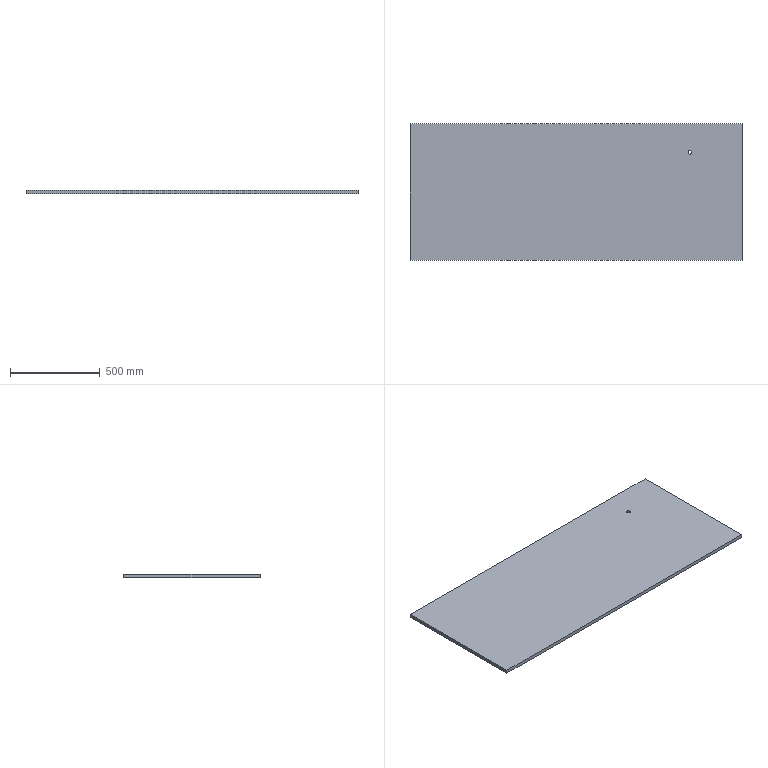Part | SolidWorks | features Extrusion 1 | 1 solid | 8 faces | box 1845 x 760 x 20 mm | volume 28037717 mm3 | plane 6 | cylinder 2 | commonest cylinder face diameters 20 x2
STEP:
#1=CARTESIAN_POINT('',(1545.,600.,20.));
#2=VERTEX_POINT('',#1);
#3=CARTESIAN_POINT('',(1565.,600.,20.));
#4=VERTEX_POINT('',#3);
#5=CARTESIAN_POINT('',(1555.,600.,20.));
#6=DIRECTION('',(0.,0.,1.));
#7=DIRECTION('',(1.,0.,0.));
#8=AXIS2_PLACEMENT_3D('',#5,#6,#7);
#9=CIRCLE('',#8,10.);
#10=EDGE_CURVE('',#2,#4,#9,.T.);
#11=ORIENTED_EDGE('',*,*,#10,.T.);
#12=CARTESIAN_POINT('',(1565.,600.,0.));
#13=VERTEX_POINT('',#12);
#14=CARTESIAN_POINT('',(1565.,600.,20.));
#15=DIRECTION('',(0.,0.,-1.));
#16=VECTOR('',#15,1000.);
#17=LINE('',#14,#16);
#18=EDGE_CURVE('',#4,#13,#17,.T.);
#19=ORIENTED_EDGE('',*,*,#18,.T.);
#20=CARTESIAN_POINT('',(1545.,600.,0.));
#21=VERTEX_POINT('',#20);
#22=CARTESIAN_POINT('',(1555.,600.,0.));
#23=DIRECTION('',(0.,0.,1.));
#24=DIRECTION('',(1.,0.,0.));
#25=AXIS2_PLACEMENT_3D('',#22,#23,#24);
#26=CIRCLE('',#25,10.);
#27=EDGE_CURVE('',#21,#13,#26,.T.);
#28=ORIENTED_EDGE('',*,*,#27,.F.);
#29=CARTESIAN_POINT('',(1545.,600.,20.));
#30=DIRECTION('',(0.,0.,-1.));
#31=VECTOR('',#30,1000.);
#32=LINE('',#29,#31);
#33=EDGE_CURVE('',#2,#21,#32,.T.);
#34=ORIENTED_EDGE('',*,*,#33,.F.);
#35=EDGE_LOOP('',(#11,#19,#28,#34));
#36=FACE_OUTER_BOUND('',#35,.T.);
#37=CARTESIAN_POINT('',(1555.,600.,20.));
#38=DIRECTION('',(0.,0.,-1.));
#39=DIRECTION('',(-1.,0.,0.));
#40=AXIS2_PLACEMENT_3D('',#37,#38,#39);
#41=CYLINDRICAL_SURFACE('',#40,10.);
#42=ADVANCED_FACE('',(#36),#41,.F.);
#43=CARTESIAN_POINT('',(0.,760.,20.));
#44=VERTEX_POINT('',#43);
#45=CARTESIAN_POINT('',(0.,0.,20.));
#46=VERTEX_POINT('',#45);
#47=CARTESIAN_POINT('',(0.,0.,20.));
#48=DIRECTION('',(0.,-1.,0.));
#49=VECTOR('',#48,1000.);
#50=LINE('',#47,#49);
#51=EDGE_CURVE('',#44,#46,#50,.T.);
#52=ORIENTED_EDGE('',*,*,#51,.T.);
#53=CARTESIAN_POINT('',(1845.,0.,20.));
#54=VERTEX_POINT('',#53);
#55=CARTESIAN_POINT('',(0.,0.,20.));
#56=DIRECTION('',(1.,0.,0.));
#57=VECTOR('',#56,1000.);
#58=LINE('',#55,#57);
#59=EDGE_CURVE('',#46,#54,#58,.T.);
#60=ORIENTED_EDGE('',*,*,#59,.T.);
#61=CARTESIAN_POINT('',(1845.,760.,20.));
#62=VERTEX_POINT('',#61);
#63=CARTESIAN_POINT('',(1845.,0.,20.));
#64=DIRECTION('',(0.,1.,0.));
#65=VECTOR('',#64,1000.);
#66=LINE('',#63,#65);
#67=EDGE_CURVE('',#54,#62,#66,.T.);
#68=ORIENTED_EDGE('',*,*,#67,.T.);
#69=CARTESIAN_POINT('',(0.,760.,20.));
#70=DIRECTION('',(-1.,0.,0.));
#71=VECTOR('',#70,1000.);
#72=LINE('',#69,#71);
#73=EDGE_CURVE('',#62,#44,#72,.T.);
#74=ORIENTED_EDGE('',*,*,#73,.T.);
#75=EDGE_LOOP('',(#52,#60,#68,#74));
#76=FACE_OUTER_BOUND('',#75,.T.);
#77=ORIENTED_EDGE('',*,*,#10,.F.);
#78=CARTESIAN_POINT('',(1555.,600.,20.));
#79=DIRECTION('',(0.,0.,1.));
#80=DIRECTION('',(1.,0.,0.));
#81=AXIS2_PLACEMENT_3D('',#78,#79,#80);
#82=CIRCLE('',#81,10.);
#83=EDGE_CURVE('',#4,#2,#82,.T.);
#84=ORIENTED_EDGE('',*,*,#83,.F.);
#85=EDGE_LOOP('',(#77,#84));
#86=FACE_BOUND('',#85,.T.);
#87=CARTESIAN_POINT('',(0.,0.,20.));
#88=DIRECTION('',(0.,0.,-1.));
#89=DIRECTION('',(-1.,0.,0.));
#90=AXIS2_PLACEMENT_3D('',#87,#88,#89);
#91=PLANE('',#90);
#92=ADVANCED_FACE('',(#76,#86),#91,.F.);
#93=CARTESIAN_POINT('',(0.,760.,0.));
#94=VERTEX_POINT('',#93);
#95=CARTESIAN_POINT('',(0.,0.,0.));
#96=VERTEX_POINT('',#95);
#97=CARTESIAN_POINT('',(0.,0.,0.));
#98=DIRECTION('',(0.,-1.,0.));
#99=VECTOR('',#98,1000.);
#100=LINE('',#97,#99);
#101=EDGE_CURVE('',#94,#96,#100,.T.);
#102=ORIENTED_EDGE('',*,*,#101,.F.);
#103=CARTESIAN_POINT('',(1845.,760.,0.));
#104=VERTEX_POINT('',#103);
#105=CARTESIAN_POINT('',(0.,760.,0.));
#106=DIRECTION('',(-1.,0.,0.));
#107=VECTOR('',#106,1000.);
#108=LINE('',#105,#107);
#109=EDGE_CURVE('',#104,#94,#108,.T.);
#110=ORIENTED_EDGE('',*,*,#109,.F.);
#111=CARTESIAN_POINT('',(1845.,0.,0.));
#112=VERTEX_POINT('',#111);
#113=CARTESIAN_POINT('',(1845.,0.,0.));
#114=DIRECTION('',(0.,1.,0.));
#115=VECTOR('',#114,1000.);
#116=LINE('',#113,#115);
#117=EDGE_CURVE('',#112,#104,#116,.T.);
#118=ORIENTED_EDGE('',*,*,#117,.F.);
#119=CARTESIAN_POINT('',(0.,0.,0.));
#120=DIRECTION('',(1.,0.,0.));
#121=VECTOR('',#120,1000.);
#122=LINE('',#119,#121);
#123=EDGE_CURVE('',#96,#112,#122,.T.);
#124=ORIENTED_EDGE('',*,*,#123,.F.);
#125=EDGE_LOOP('',(#102,#110,#118,#124));
#126=FACE_OUTER_BOUND('',#125,.T.);
#127=ORIENTED_EDGE('',*,*,#27,.T.);
#128=CARTESIAN_POINT('',(1555.,600.,0.));
#129=DIRECTION('',(0.,0.,1.));
#130=DIRECTION('',(1.,0.,0.));
#131=AXIS2_PLACEMENT_3D('',#128,#129,#130);
#132=CIRCLE('',#131,10.);
#133=EDGE_CURVE('',#13,#21,#132,.T.);
#134=ORIENTED_EDGE('',*,*,#133,.T.);
#135=EDGE_LOOP('',(#127,#134));
#136=FACE_BOUND('',#135,.T.);
#137=CARTESIAN_POINT('',(0.,0.,0.));
#138=DIRECTION('',(0.,0.,-1.));
#139=DIRECTION('',(-1.,0.,0.));
#140=AXIS2_PLACEMENT_3D('',#137,#138,#139);
#141=PLANE('',#140);
#142=ADVANCED_FACE('',(#126,#136),#141,.T.);
#143=ORIENTED_EDGE('',*,*,#101,.T.);
#144=CARTESIAN_POINT('',(0.,0.,20.));
#145=DIRECTION('',(0.,0.,-1.));
#146=VECTOR('',#145,1000.);
#147=LINE('',#144,#146);
#148=EDGE_CURVE('',#46,#96,#147,.T.);
#149=ORIENTED_EDGE('',*,*,#148,.F.);
#150=ORIENTED_EDGE('',*,*,#51,.F.);
#151=CARTESIAN_POINT('',(0.,760.,20.));
#152=DIRECTION('',(0.,0.,-1.));
#153=VECTOR('',#152,1000.);
#154=LINE('',#151,#153);
#155=EDGE_CURVE('',#44,#94,#154,.T.);
#156=ORIENTED_EDGE('',*,*,#155,.T.);
#157=EDGE_LOOP('',(#143,#149,#150,#156));
#158=FACE_OUTER_BOUND('',#157,.T.);
#159=CARTESIAN_POINT('',(0.,0.,20.));
#160=DIRECTION('',(1.,0.,0.));
#161=DIRECTION('',(0.,0.,-1.));
#162=AXIS2_PLACEMENT_3D('',#159,#160,#161);
#163=PLANE('',#162);
#164=ADVANCED_FACE('',(#158),#163,.F.);
#165=ORIENTED_EDGE('',*,*,#123,.T.);
#166=CARTESIAN_POINT('',(1845.,0.,20.));
#167=DIRECTION('',(0.,0.,-1.));
#168=VECTOR('',#167,1000.);
#169=LINE('',#166,#168);
#170=EDGE_CURVE('',#54,#112,#169,.T.);
#171=ORIENTED_EDGE('',*,*,#170,.F.);
#172=ORIENTED_EDGE('',*,*,#59,.F.);
#173=ORIENTED_EDGE('',*,*,#148,.T.);
#174=EDGE_LOOP('',(#165,#171,#172,#173));
#175=FACE_OUTER_BOUND('',#174,.T.);
#176=CARTESIAN_POINT('',(0.,0.,20.));
#177=DIRECTION('',(0.,1.,0.));
#178=DIRECTION('',(0.,0.,1.));
#179=AXIS2_PLACEMENT_3D('',#176,#177,#178);
#180=PLANE('',#179);
#181=ADVANCED_FACE('',(#175),#180,.F.);
#182=ORIENTED_EDGE('',*,*,#117,.T.);
#183=CARTESIAN_POINT('',(1845.,760.,20.));
#184=DIRECTION('',(0.,0.,-1.));
#185=VECTOR('',#184,1000.);
#186=LINE('',#183,#185);
#187=EDGE_CURVE('',#62,#104,#186,.T.);
#188=ORIENTED_EDGE('',*,*,#187,.F.);
#189=ORIENTED_EDGE('',*,*,#67,.F.);
#190=ORIENTED_EDGE('',*,*,#170,.T.);
#191=EDGE_LOOP('',(#182,#188,#189,#190));
#192=FACE_OUTER_BOUND('',#191,.T.);
#193=CARTESIAN_POINT('',(1845.,0.,20.));
#194=DIRECTION('',(-1.,0.,0.));
#195=DIRECTION('',(0.,0.,1.));
#196=AXIS2_PLACEMENT_3D('',#193,#194,#195);
#197=PLANE('',#196);
#198=ADVANCED_FACE('',(#192),#197,.F.);
#199=ORIENTED_EDGE('',*,*,#109,.T.);
#200=ORIENTED_EDGE('',*,*,#155,.F.);
#201=ORIENTED_EDGE('',*,*,#73,.F.);
#202=ORIENTED_EDGE('',*,*,#187,.T.);
#203=EDGE_LOOP('',(#199,#200,#201,#202));
#204=FACE_OUTER_BOUND('',#203,.T.);
#205=CARTESIAN_POINT('',(0.,760.,20.));
#206=DIRECTION('',(0.,-1.,0.));
#207=DIRECTION('',(0.,0.,-1.));
#208=AXIS2_PLACEMENT_3D('',#205,#206,#207);
#209=PLANE('',#208);
#210=ADVANCED_FACE('',(#204),#209,.F.);
#211=ORIENTED_EDGE('',*,*,#18,.F.);
#212=ORIENTED_EDGE('',*,*,#83,.T.);
#213=ORIENTED_EDGE('',*,*,#33,.T.);
#214=ORIENTED_EDGE('',*,*,#133,.F.);
#215=EDGE_LOOP('',(#211,#212,#213,#214));
#216=FACE_OUTER_BOUND('',#215,.T.);
#217=CARTESIAN_POINT('',(1555.,600.,20.));
#218=DIRECTION('',(0.,0.,-1.));
#219=DIRECTION('',(-1.,0.,0.));
#220=AXIS2_PLACEMENT_3D('',#217,#218,#219);
#221=CYLINDRICAL_SURFACE('',#220,10.);
#222=ADVANCED_FACE('',(#216),#221,.F.);
#223=CLOSED_SHELL('',(#42,#92,#142,#164,#181,#198,#210,#222));
#224=MANIFOLD_SOLID_BREP('',#223);
#225=CARTESIAN_POINT('',(0.,0.,0.));
#226=DIRECTION('',(0.,0.,1.));
#227=DIRECTION('',(1.,0.,0.));
#228=AXIS2_PLACEMENT_3D('',#225,#226,#227);
#229=(LENGTH_UNIT()NAMED_UNIT(*)SI_UNIT(.MILLI.,.METRE.));
#230=UNCERTAINTY_MEASURE_WITH_UNIT(LENGTH_MEASURE(0.00001),#229,'','');
#231=(NAMED_UNIT(*)PLANE_ANGLE_UNIT()SI_UNIT($,.RADIAN.));
#232=(NAMED_UNIT(*)SI_UNIT($,.STERADIAN.)SOLID_ANGLE_UNIT());
#233=(GEOMETRIC_REPRESENTATION_CONTEXT(3)GLOBAL_UNCERTAINTY_ASSIGNED_CONTEXT((#230))GLOBAL_UNIT_ASSIGNED_CONTEXT((#229,#231,#232))REPRESENTATION_CONTEXT('',''));
#234=ADVANCED_BREP_SHAPE_REPRESENTATION('',(#224,#228),#233);